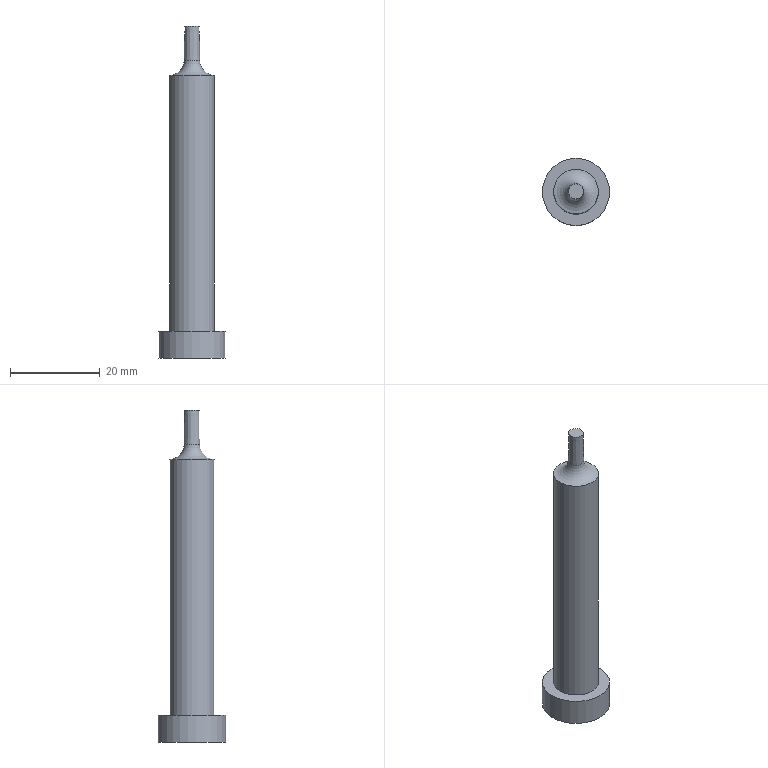Part | STEP file | solid 63 | 1 solid | 7 faces | box 15 x 15 x 74.066 mm | volume 5678 mm3 | plane 3 | cylinder 2 | cone 1 | torus 1 | commonest cylinder face diameters 10 x1 15 x1